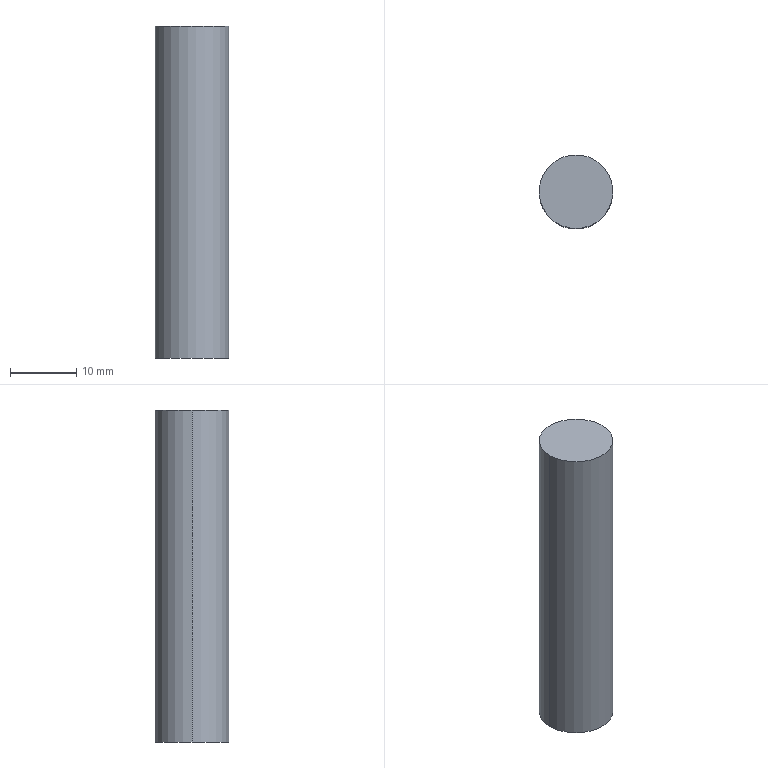Part | STEP file | 4-20.sldasm-Part-343 | 1 solid | 4 faces | box 11.11 x 11.11 x 50 mm | volume 4847 mm3 | cylinder 2 | plane 2 | commonest cylinder face diameters 11.11 x2
STEP:
#1=CARTESIAN_POINT('',(-44.445,380.,90.));
#2=VERTEX_POINT('',#1);
#3=CARTESIAN_POINT('',(-55.555,380.,90.));
#4=VERTEX_POINT('',#3);
#5=CARTESIAN_POINT('',(-50.,380.,90.));
#6=DIRECTION('',(0.,0.,-1.));
#7=DIRECTION('',(1.,0.,0.));
#8=AXIS2_PLACEMENT_3D('',#5,#6,#7);
#9=CIRCLE('',#8,5.555);
#10=EDGE_CURVE('',#2,#4,#9,.T.);
#11=ORIENTED_EDGE('',*,*,#10,.T.);
#12=CARTESIAN_POINT('',(-55.555,380.,40.));
#13=VERTEX_POINT('',#12);
#14=CARTESIAN_POINT('',(-55.555,380.,-10.));
#15=DIRECTION('',(0.,0.,-1.));
#16=VECTOR('',#15,1000.);
#17=LINE('',#14,#16);
#18=EDGE_CURVE('',#4,#13,#17,.T.);
#19=ORIENTED_EDGE('',*,*,#18,.T.);
#20=CARTESIAN_POINT('',(-44.445,380.,40.));
#21=VERTEX_POINT('',#20);
#22=CARTESIAN_POINT('',(-50.,380.,40.));
#23=DIRECTION('',(0.,0.,1.));
#24=DIRECTION('',(-1.,0.,0.));
#25=AXIS2_PLACEMENT_3D('',#22,#23,#24);
#26=CIRCLE('',#25,5.555);
#27=EDGE_CURVE('',#13,#21,#26,.T.);
#28=ORIENTED_EDGE('',*,*,#27,.T.);
#29=CARTESIAN_POINT('',(-44.445,380.,-10.));
#30=DIRECTION('',(0.,0.,-1.));
#31=VECTOR('',#30,1000.);
#32=LINE('',#29,#31);
#33=EDGE_CURVE('',#2,#21,#32,.T.);
#34=ORIENTED_EDGE('',*,*,#33,.F.);
#35=EDGE_LOOP('',(#11,#19,#28,#34));
#36=FACE_OUTER_BOUND('',#35,.T.);
#37=CARTESIAN_POINT('',(-50.,380.,-10.));
#38=DIRECTION('',(0.,0.,-1.));
#39=DIRECTION('',(1.,0.,0.));
#40=AXIS2_PLACEMENT_3D('',#37,#38,#39);
#41=CYLINDRICAL_SURFACE('',#40,5.555);
#42=ADVANCED_FACE('',(#36),#41,.T.);
#43=ORIENTED_EDGE('',*,*,#18,.F.);
#44=CARTESIAN_POINT('',(-50.,380.,90.));
#45=DIRECTION('',(0.,0.,-1.));
#46=DIRECTION('',(1.,0.,0.));
#47=AXIS2_PLACEMENT_3D('',#44,#45,#46);
#48=CIRCLE('',#47,5.555);
#49=EDGE_CURVE('',#4,#2,#48,.T.);
#50=ORIENTED_EDGE('',*,*,#49,.T.);
#51=ORIENTED_EDGE('',*,*,#33,.T.);
#52=CARTESIAN_POINT('',(-50.,380.,40.));
#53=DIRECTION('',(0.,0.,1.));
#54=DIRECTION('',(-1.,0.,0.));
#55=AXIS2_PLACEMENT_3D('',#52,#53,#54);
#56=CIRCLE('',#55,5.555);
#57=EDGE_CURVE('',#21,#13,#56,.T.);
#58=ORIENTED_EDGE('',*,*,#57,.T.);
#59=EDGE_LOOP('',(#43,#50,#51,#58));
#60=FACE_OUTER_BOUND('',#59,.T.);
#61=CARTESIAN_POINT('',(-50.,380.,-10.));
#62=DIRECTION('',(0.,0.,-1.));
#63=DIRECTION('',(1.,0.,0.));
#64=AXIS2_PLACEMENT_3D('',#61,#62,#63);
#65=CYLINDRICAL_SURFACE('',#64,5.555);
#66=ADVANCED_FACE('',(#60),#65,.T.);
#67=ORIENTED_EDGE('',*,*,#10,.F.);
#68=ORIENTED_EDGE('',*,*,#49,.F.);
#69=EDGE_LOOP('',(#67,#68));
#70=FACE_OUTER_BOUND('',#69,.T.);
#71=CARTESIAN_POINT('',(-50.,380.,90.));
#72=DIRECTION('',(0.,0.,1.));
#73=DIRECTION('',(-1.,0.,0.));
#74=AXIS2_PLACEMENT_3D('',#71,#72,#73);
#75=PLANE('',#74);
#76=ADVANCED_FACE('',(#70),#75,.T.);
#77=ORIENTED_EDGE('',*,*,#57,.F.);
#78=ORIENTED_EDGE('',*,*,#27,.F.);
#79=EDGE_LOOP('',(#77,#78));
#80=FACE_OUTER_BOUND('',#79,.T.);
#81=CARTESIAN_POINT('',(100.,10.,40.));
#82=DIRECTION('',(0.,0.,-1.));
#83=DIRECTION('',(-1.,0.,0.));
#84=AXIS2_PLACEMENT_3D('',#81,#82,#83);
#85=PLANE('',#84);
#86=ADVANCED_FACE('',(#80),#85,.T.);
#87=CLOSED_SHELL('',(#42,#66,#76,#86));
#88=MANIFOLD_SOLID_BREP('',#87);
#89=CARTESIAN_POINT('',(0.,0.,0.));
#90=DIRECTION('',(0.,0.,1.));
#91=DIRECTION('',(1.,0.,0.));
#92=AXIS2_PLACEMENT_3D('',#89,#90,#91);
#93=(LENGTH_UNIT()NAMED_UNIT(*)SI_UNIT(.MILLI.,.METRE.));
#94=UNCERTAINTY_MEASURE_WITH_UNIT(LENGTH_MEASURE(0.00001),#93,'','');
#95=(NAMED_UNIT(*)PLANE_ANGLE_UNIT()SI_UNIT($,.RADIAN.));
#96=(NAMED_UNIT(*)SI_UNIT($,.STERADIAN.)SOLID_ANGLE_UNIT());
#97=(GEOMETRIC_REPRESENTATION_CONTEXT(3)GLOBAL_UNCERTAINTY_ASSIGNED_CONTEXT((#94))GLOBAL_UNIT_ASSIGNED_CONTEXT((#93,#95,#96))REPRESENTATION_CONTEXT('',''));
#98=ADVANCED_BREP_SHAPE_REPRESENTATION('',(#88,#92),#97);